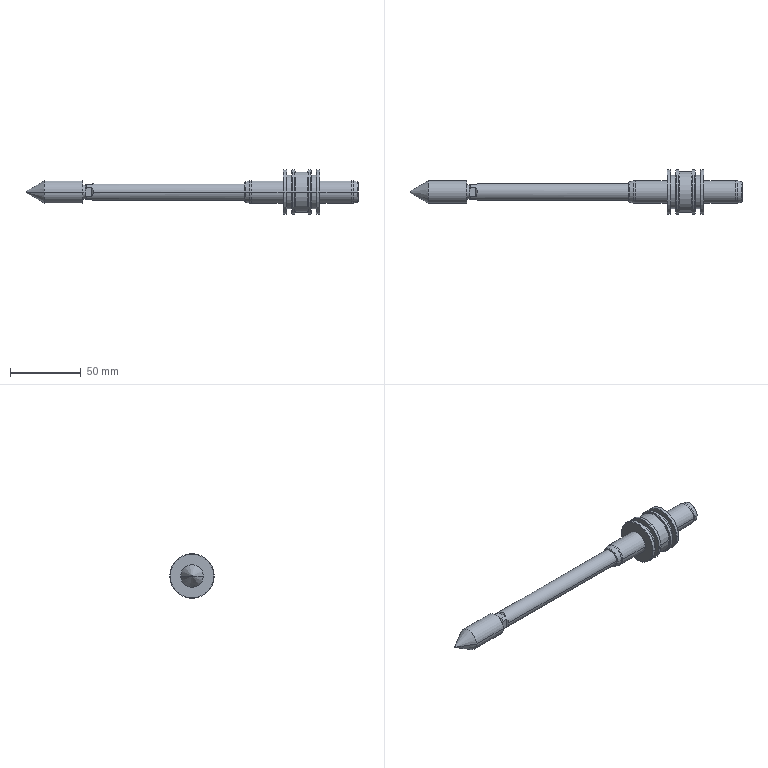Part | STEP file | 1 solid | 87 faces | box 235 x 31.5 x 31.5 mm | volume 41265 mm3 | cone 30 | cylinder 24 | plane 21 | torus 8 | other 4 | commonest cylinder face diameters 31.5 x8 16 x6 24 x4 10 x2 12 x2 28.9 x2